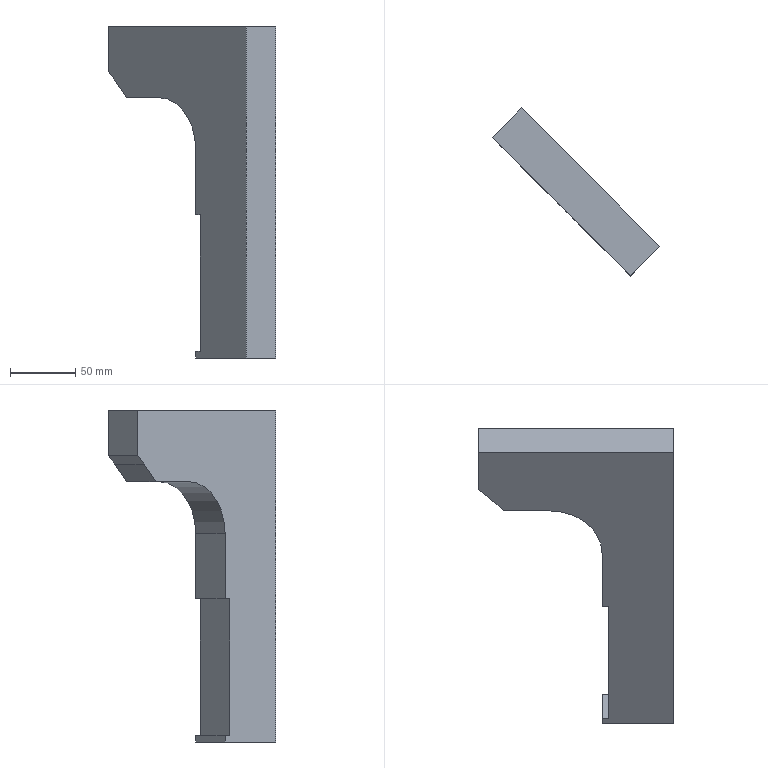Part | NX | features solid 2 | 1 solid | 15 faces | box 128.693 x 128.693 x 255 mm | volume 603628 mm3 | plane 14 | cylinder 1 | commonest cylinder face diameters 80 x1
STEP:
#1=CARTESIAN_POINT('',(803.273,-568.514,15.));
#2=VERTEX_POINT('',#1);
#3=CARTESIAN_POINT('',(803.273,-568.514,50.));
#4=VERTEX_POINT('',#3);
#5=CARTESIAN_POINT('',(803.273,-568.514,15.));
#6=DIRECTION('',(0.,0.,1.));
#7=VECTOR('',#6,1000.);
#8=LINE('',#5,#7);
#9=EDGE_CURVE('',#2,#4,#8,.T.);
#10=ORIENTED_EDGE('',*,*,#9,.F.);
#11=CARTESIAN_POINT('',(780.646,-591.141,15.));
#12=VERTEX_POINT('',#11);
#13=CARTESIAN_POINT('',(780.646,-591.141,15.));
#14=DIRECTION('',(0.7071,0.7071,0.));
#15=VECTOR('',#14,1000.);
#16=LINE('',#13,#15);
#17=EDGE_CURVE('',#12,#2,#16,.T.);
#18=ORIENTED_EDGE('',*,*,#17,.F.);
#19=CARTESIAN_POINT('',(780.646,-591.141,50.));
#20=VERTEX_POINT('',#19);
#21=CARTESIAN_POINT('',(780.646,-591.141,15.));
#22=DIRECTION('',(0.,0.,1.));
#23=VECTOR('',#22,1000.);
#24=LINE('',#21,#23);
#25=EDGE_CURVE('',#12,#20,#24,.T.);
#26=ORIENTED_EDGE('',*,*,#25,.T.);
#27=CARTESIAN_POINT('',(780.646,-591.141,50.));
#28=DIRECTION('',(0.7071,0.7071,0.));
#29=VECTOR('',#28,1000.);
#30=LINE('',#27,#29);
#31=EDGE_CURVE('',#20,#4,#30,.T.);
#32=ORIENTED_EDGE('',*,*,#31,.T.);
#33=EDGE_LOOP('',(#10,#18,#26,#32));
#34=FACE_BOUND('',#33,.T.);
#35=CARTESIAN_POINT('',(780.646,-591.141,15.));
#36=DIRECTION('',(-0.7071,0.7071,0.));
#37=DIRECTION('',(0.,0.,-1.));
#38=AXIS2_PLACEMENT_3D('',#35,#36,#37);
#39=PLANE('',#38);
#40=ADVANCED_FACE('',(#34),#39,.T.);
#41=CARTESIAN_POINT('',(808.223,-573.464,8.5));
#42=VERTEX_POINT('',#41);
#43=CARTESIAN_POINT('',(803.273,-568.514,15.));
#44=DIRECTION('',(0.5182,-0.5182,-0.6805));
#45=VECTOR('',#44,1000.);
#46=LINE('',#43,#45);
#47=EDGE_CURVE('',#2,#42,#46,.T.);
#48=ORIENTED_EDGE('',*,*,#47,.T.);
#49=CARTESIAN_POINT('',(785.596,-596.091,8.5));
#50=VERTEX_POINT('',#49);
#51=CARTESIAN_POINT('',(785.596,-596.091,8.5));
#52=DIRECTION('',(0.7071,0.7071,0.));
#53=VECTOR('',#52,1000.);
#54=LINE('',#51,#53);
#55=EDGE_CURVE('',#50,#42,#54,.T.);
#56=ORIENTED_EDGE('',*,*,#55,.F.);
#57=CARTESIAN_POINT('',(780.646,-591.141,15.));
#58=DIRECTION('',(0.5182,-0.5182,-0.6805));
#59=VECTOR('',#58,1000.);
#60=LINE('',#57,#59);
#61=EDGE_CURVE('',#12,#50,#60,.T.);
#62=ORIENTED_EDGE('',*,*,#61,.F.);
#63=ORIENTED_EDGE('',*,*,#17,.T.);
#64=EDGE_LOOP('',(#48,#56,#62,#63));
#65=FACE_BOUND('',#64,.T.);
#66=CARTESIAN_POINT('',(780.646,-591.141,15.));
#67=DIRECTION('',(0.4812,-0.4812,0.7328));
#68=DIRECTION('',(-0.5182,0.5182,0.6805));
#69=AXIS2_PLACEMENT_3D('',#66,#67,#68);
#70=PLANE('',#69);
#71=ADVANCED_FACE('',(#65),#70,.F.);
#72=CARTESIAN_POINT('',(817.415,-582.656,-5.));
#73=VERTEX_POINT('',#72);
#74=CARTESIAN_POINT('',(808.223,-573.464,8.5));
#75=DIRECTION('',(0.4905,-0.4905,-0.7203));
#76=VECTOR('',#75,1000.);
#77=LINE('',#74,#76);
#78=EDGE_CURVE('',#42,#73,#77,.T.);
#79=ORIENTED_EDGE('',*,*,#78,.T.);
#80=CARTESIAN_POINT('',(794.788,-605.283,-5.));
#81=VERTEX_POINT('',#80);
#82=CARTESIAN_POINT('',(794.788,-605.283,-5.));
#83=DIRECTION('',(0.7071,0.7071,0.));
#84=VECTOR('',#83,1000.);
#85=LINE('',#82,#84);
#86=EDGE_CURVE('',#81,#73,#85,.T.);
#87=ORIENTED_EDGE('',*,*,#86,.F.);
#88=CARTESIAN_POINT('',(785.596,-596.091,8.5));
#89=DIRECTION('',(0.4905,-0.4905,-0.7203));
#90=VECTOR('',#89,1000.);
#91=LINE('',#88,#90);
#92=EDGE_CURVE('',#50,#81,#91,.T.);
#93=ORIENTED_EDGE('',*,*,#92,.F.);
#94=ORIENTED_EDGE('',*,*,#55,.T.);
#95=EDGE_LOOP('',(#79,#87,#93,#94));
#96=FACE_BOUND('',#95,.T.);
#97=CARTESIAN_POINT('',(785.596,-596.091,8.5));
#98=DIRECTION('',(0.5093,-0.5093,0.6936));
#99=DIRECTION('',(-0.4905,0.4905,0.7203));
#100=AXIS2_PLACEMENT_3D('',#97,#98,#99);
#101=PLANE('',#100);
#102=ADVANCED_FACE('',(#96),#101,.F.);
#103=CARTESIAN_POINT('',(842.164,-607.405,-5.));
#104=VERTEX_POINT('',#103);
#105=CARTESIAN_POINT('',(817.415,-582.656,-5.));
#106=DIRECTION('',(0.7071,-0.7071,0.));
#107=VECTOR('',#106,1000.);
#108=LINE('',#105,#107);
#109=EDGE_CURVE('',#73,#104,#108,.T.);
#110=ORIENTED_EDGE('',*,*,#109,.T.);
#111=CARTESIAN_POINT('',(819.537,-630.032,-5.));
#112=VERTEX_POINT('',#111);
#113=CARTESIAN_POINT('',(819.537,-630.032,-5.));
#114=DIRECTION('',(0.7071,0.7071,0.));
#115=VECTOR('',#114,1000.);
#116=LINE('',#113,#115);
#117=EDGE_CURVE('',#112,#104,#116,.T.);
#118=ORIENTED_EDGE('',*,*,#117,.F.);
#119=CARTESIAN_POINT('',(794.788,-605.283,-5.));
#120=DIRECTION('',(0.7071,-0.7071,0.));
#121=VECTOR('',#120,1000.);
#122=LINE('',#119,#121);
#123=EDGE_CURVE('',#81,#112,#122,.T.);
#124=ORIENTED_EDGE('',*,*,#123,.F.);
#125=ORIENTED_EDGE('',*,*,#86,.T.);
#126=EDGE_LOOP('',(#110,#118,#124,#125));
#127=FACE_BOUND('',#126,.T.);
#128=CARTESIAN_POINT('',(794.788,-605.283,-5.));
#129=DIRECTION('',(0.,0.,1.));
#130=DIRECTION('',(-0.7071,0.7071,0.));
#131=AXIS2_PLACEMENT_3D('',#128,#129,#130);
#132=PLANE('',#131);
#133=ADVANCED_FACE('',(#127),#132,.F.);
#134=CARTESIAN_POINT('',(870.448,-635.689,-45.));
#135=VERTEX_POINT('',#134);
#136=CARTESIAN_POINT('',(842.164,-607.405,-45.));
#137=DIRECTION('',(-0.7071,-0.7071,0.));
#138=DIRECTION('',(0.7071,-0.7071,0.));
#139=AXIS2_PLACEMENT_3D('',#136,#137,#138);
#140=CIRCLE('',#139,40.);
#141=EDGE_CURVE('',#135,#104,#140,.T.);
#142=ORIENTED_EDGE('',*,*,#141,.F.);
#143=CARTESIAN_POINT('',(847.821,-658.316,-45.));
#144=VERTEX_POINT('',#143);
#145=CARTESIAN_POINT('',(847.821,-658.316,-45.));
#146=DIRECTION('',(0.7071,0.7071,0.));
#147=VECTOR('',#146,1000.);
#148=LINE('',#145,#147);
#149=EDGE_CURVE('',#144,#135,#148,.T.);
#150=ORIENTED_EDGE('',*,*,#149,.F.);
#151=CARTESIAN_POINT('',(819.537,-630.032,-45.));
#152=DIRECTION('',(-0.7071,-0.7071,0.));
#153=DIRECTION('',(0.7071,-0.7071,0.));
#154=AXIS2_PLACEMENT_3D('',#151,#152,#153);
#155=CIRCLE('',#154,40.);
#156=EDGE_CURVE('',#144,#112,#155,.T.);
#157=ORIENTED_EDGE('',*,*,#156,.T.);
#158=ORIENTED_EDGE('',*,*,#117,.T.);
#159=EDGE_LOOP('',(#142,#150,#157,#158));
#160=FACE_BOUND('',#159,.T.);
#161=CARTESIAN_POINT('',(819.537,-630.032,-45.));
#162=DIRECTION('',(0.7071,0.7071,0.));
#163=DIRECTION('',(0.,0.,-1.));
#164=AXIS2_PLACEMENT_3D('',#161,#162,#163);
#165=CYLINDRICAL_SURFACE('',#164,40.);
#166=ADVANCED_FACE('',(#160),#165,.F.);
#167=CARTESIAN_POINT('',(870.448,-635.689,-95.));
#168=VERTEX_POINT('',#167);
#169=CARTESIAN_POINT('',(870.448,-635.689,-45.));
#170=DIRECTION('',(0.,0.,-1.));
#171=VECTOR('',#170,1000.);
#172=LINE('',#169,#171);
#173=EDGE_CURVE('',#135,#168,#172,.T.);
#174=ORIENTED_EDGE('',*,*,#173,.T.);
#175=CARTESIAN_POINT('',(847.821,-658.316,-95.));
#176=VERTEX_POINT('',#175);
#177=CARTESIAN_POINT('',(847.821,-658.316,-95.));
#178=DIRECTION('',(0.7071,0.7071,0.));
#179=VECTOR('',#178,1000.);
#180=LINE('',#177,#179);
#181=EDGE_CURVE('',#176,#168,#180,.T.);
#182=ORIENTED_EDGE('',*,*,#181,.F.);
#183=CARTESIAN_POINT('',(847.821,-658.316,-45.));
#184=DIRECTION('',(0.,0.,-1.));
#185=VECTOR('',#184,1000.);
#186=LINE('',#183,#185);
#187=EDGE_CURVE('',#144,#176,#186,.T.);
#188=ORIENTED_EDGE('',*,*,#187,.F.);
#189=ORIENTED_EDGE('',*,*,#149,.T.);
#190=EDGE_LOOP('',(#174,#182,#188,#189));
#191=FACE_BOUND('',#190,.T.);
#192=CARTESIAN_POINT('',(847.821,-658.316,-45.));
#193=DIRECTION('',(0.7071,-0.7071,0.));
#194=DIRECTION('',(0.,0.,1.));
#195=AXIS2_PLACEMENT_3D('',#192,#193,#194);
#196=PLANE('',#195);
#197=ADVANCED_FACE('',(#191),#196,.F.);
#198=CARTESIAN_POINT('',(873.984,-639.225,-95.));
#199=VERTEX_POINT('',#198);
#200=CARTESIAN_POINT('',(863.377,-628.618,-95.));
#201=DIRECTION('',(0.7071,-0.7071,0.));
#202=VECTOR('',#201,1000.);
#203=LINE('',#200,#202);
#204=EDGE_CURVE('',#168,#199,#203,.T.);
#205=ORIENTED_EDGE('',*,*,#204,.T.);
#206=CARTESIAN_POINT('',(851.357,-661.852,-95.));
#207=VERTEX_POINT('',#206);
#208=CARTESIAN_POINT('',(851.357,-661.852,-95.));
#209=DIRECTION('',(0.7071,0.7071,0.));
#210=VECTOR('',#209,1000.);
#211=LINE('',#208,#210);
#212=EDGE_CURVE('',#207,#199,#211,.T.);
#213=ORIENTED_EDGE('',*,*,#212,.F.);
#214=CARTESIAN_POINT('',(840.75,-651.245,-95.));
#215=DIRECTION('',(0.7071,-0.7071,0.));
#216=VECTOR('',#215,1000.);
#217=LINE('',#214,#216);
#218=EDGE_CURVE('',#176,#207,#217,.T.);
#219=ORIENTED_EDGE('',*,*,#218,.F.);
#220=ORIENTED_EDGE('',*,*,#181,.T.);
#221=EDGE_LOOP('',(#205,#213,#219,#220));
#222=FACE_BOUND('',#221,.T.);
#223=CARTESIAN_POINT('',(840.75,-651.245,-95.));
#224=DIRECTION('',(0.,0.,1.));
#225=DIRECTION('',(-0.7071,0.7071,0.));
#226=AXIS2_PLACEMENT_3D('',#223,#224,#225);
#227=PLANE('',#226);
#228=ADVANCED_FACE('',(#222),#227,.F.);
#229=CARTESIAN_POINT('',(873.984,-639.225,-200.));
#230=VERTEX_POINT('',#229);
#231=CARTESIAN_POINT('',(873.984,-639.225,-95.));
#232=DIRECTION('',(0.,0.,-1.));
#233=VECTOR('',#232,1000.);
#234=LINE('',#231,#233);
#235=EDGE_CURVE('',#199,#230,#234,.T.);
#236=ORIENTED_EDGE('',*,*,#235,.T.);
#237=CARTESIAN_POINT('',(851.357,-661.852,-200.));
#238=VERTEX_POINT('',#237);
#239=CARTESIAN_POINT('',(851.357,-661.852,-200.));
#240=DIRECTION('',(0.7071,0.7071,0.));
#241=VECTOR('',#240,1000.);
#242=LINE('',#239,#241);
#243=EDGE_CURVE('',#238,#230,#242,.T.);
#244=ORIENTED_EDGE('',*,*,#243,.F.);
#245=CARTESIAN_POINT('',(851.357,-661.852,-95.));
#246=DIRECTION('',(0.,0.,-1.));
#247=VECTOR('',#246,1000.);
#248=LINE('',#245,#247);
#249=EDGE_CURVE('',#207,#238,#248,.T.);
#250=ORIENTED_EDGE('',*,*,#249,.F.);
#251=ORIENTED_EDGE('',*,*,#212,.T.);
#252=EDGE_LOOP('',(#236,#244,#250,#251));
#253=FACE_BOUND('',#252,.T.);
#254=CARTESIAN_POINT('',(851.357,-661.852,-95.));
#255=DIRECTION('',(0.7071,-0.7071,0.));
#256=DIRECTION('',(0.,0.,1.));
#257=AXIS2_PLACEMENT_3D('',#254,#255,#256);
#258=PLANE('',#257);
#259=ADVANCED_FACE('',(#253),#258,.F.);
#260=CARTESIAN_POINT('',(870.448,-635.689,-200.));
#261=VERTEX_POINT('',#260);
#262=CARTESIAN_POINT('',(873.984,-639.225,-200.));
#263=DIRECTION('',(-0.7071,0.7071,0.));
#264=VECTOR('',#263,1000.);
#265=LINE('',#262,#264);
#266=EDGE_CURVE('',#230,#261,#265,.T.);
#267=ORIENTED_EDGE('',*,*,#266,.T.);
#268=CARTESIAN_POINT('',(847.821,-658.316,-200.));
#269=VERTEX_POINT('',#268);
#270=CARTESIAN_POINT('',(847.821,-658.316,-200.));
#271=DIRECTION('',(0.7071,0.7071,0.));
#272=VECTOR('',#271,1000.);
#273=LINE('',#270,#272);
#274=EDGE_CURVE('',#269,#261,#273,.T.);
#275=ORIENTED_EDGE('',*,*,#274,.F.);
#276=CARTESIAN_POINT('',(851.357,-661.852,-200.));
#277=DIRECTION('',(-0.7071,0.7071,0.));
#278=VECTOR('',#277,1000.);
#279=LINE('',#276,#278);
#280=EDGE_CURVE('',#238,#269,#279,.T.);
#281=ORIENTED_EDGE('',*,*,#280,.F.);
#282=ORIENTED_EDGE('',*,*,#243,.T.);
#283=EDGE_LOOP('',(#267,#275,#281,#282));
#284=FACE_BOUND('',#283,.T.);
#285=CARTESIAN_POINT('',(851.357,-661.852,-200.));
#286=DIRECTION('',(0.,0.,-1.));
#287=DIRECTION('',(0.7071,-0.7071,0.));
#288=AXIS2_PLACEMENT_3D('',#285,#286,#287);
#289=PLANE('',#288);
#290=ADVANCED_FACE('',(#284),#289,.F.);
#291=CARTESIAN_POINT('',(870.448,-635.689,-205.));
#292=VERTEX_POINT('',#291);
#293=CARTESIAN_POINT('',(870.448,-635.689,-200.));
#294=DIRECTION('',(0.,0.,-1.));
#295=VECTOR('',#294,1000.);
#296=LINE('',#293,#295);
#297=EDGE_CURVE('',#261,#292,#296,.T.);
#298=ORIENTED_EDGE('',*,*,#297,.T.);
#299=CARTESIAN_POINT('',(847.821,-658.316,-205.));
#300=VERTEX_POINT('',#299);
#301=CARTESIAN_POINT('',(847.821,-658.316,-205.));
#302=DIRECTION('',(0.7071,0.7071,0.));
#303=VECTOR('',#302,1000.);
#304=LINE('',#301,#303);
#305=EDGE_CURVE('',#300,#292,#304,.T.);
#306=ORIENTED_EDGE('',*,*,#305,.F.);
#307=CARTESIAN_POINT('',(847.821,-658.316,-200.));
#308=DIRECTION('',(0.,0.,-1.));
#309=VECTOR('',#308,1000.);
#310=LINE('',#307,#309);
#311=EDGE_CURVE('',#269,#300,#310,.T.);
#312=ORIENTED_EDGE('',*,*,#311,.F.);
#313=ORIENTED_EDGE('',*,*,#274,.T.);
#314=EDGE_LOOP('',(#298,#306,#312,#313));
#315=FACE_BOUND('',#314,.T.);
#316=CARTESIAN_POINT('',(847.821,-658.316,-200.));
#317=DIRECTION('',(0.7071,-0.7071,0.));
#318=DIRECTION('',(0.,0.,1.));
#319=AXIS2_PLACEMENT_3D('',#316,#317,#318);
#320=PLANE('',#319);
#321=ADVANCED_FACE('',(#315),#320,.F.);
#322=CARTESIAN_POINT('',(909.339,-674.58,-205.));
#323=VERTEX_POINT('',#322);
#324=CARTESIAN_POINT('',(870.448,-635.689,-205.));
#325=DIRECTION('',(0.7071,-0.7071,0.));
#326=VECTOR('',#325,1000.);
#327=LINE('',#324,#326);
#328=EDGE_CURVE('',#292,#323,#327,.T.);
#329=ORIENTED_EDGE('',*,*,#328,.T.);
#330=CARTESIAN_POINT('',(886.712,-697.207,-205.));
#331=VERTEX_POINT('',#330);
#332=CARTESIAN_POINT('',(886.712,-697.207,-205.));
#333=DIRECTION('',(0.7071,0.7071,0.));
#334=VECTOR('',#333,1000.);
#335=LINE('',#332,#334);
#336=EDGE_CURVE('',#331,#323,#335,.T.);
#337=ORIENTED_EDGE('',*,*,#336,.F.);
#338=CARTESIAN_POINT('',(847.821,-658.316,-205.));
#339=DIRECTION('',(0.7071,-0.7071,0.));
#340=VECTOR('',#339,1000.);
#341=LINE('',#338,#340);
#342=EDGE_CURVE('',#300,#331,#341,.T.);
#343=ORIENTED_EDGE('',*,*,#342,.F.);
#344=ORIENTED_EDGE('',*,*,#305,.T.);
#345=EDGE_LOOP('',(#329,#337,#343,#344));
#346=FACE_BOUND('',#345,.T.);
#347=CARTESIAN_POINT('',(847.821,-658.316,-205.));
#348=DIRECTION('',(0.,0.,1.));
#349=DIRECTION('',(-0.7071,0.7071,0.));
#350=AXIS2_PLACEMENT_3D('',#347,#348,#349);
#351=PLANE('',#350);
#352=ADVANCED_FACE('',(#346),#351,.F.);
#353=CARTESIAN_POINT('',(909.339,-674.58,50.));
#354=VERTEX_POINT('',#353);
#355=CARTESIAN_POINT('',(909.339,-674.58,-205.));
#356=DIRECTION('',(0.,0.,1.));
#357=VECTOR('',#356,1000.);
#358=LINE('',#355,#357);
#359=EDGE_CURVE('',#323,#354,#358,.T.);
#360=ORIENTED_EDGE('',*,*,#359,.T.);
#361=CARTESIAN_POINT('',(886.712,-697.207,50.));
#362=VERTEX_POINT('',#361);
#363=CARTESIAN_POINT('',(886.712,-697.207,50.));
#364=DIRECTION('',(0.7071,0.7071,0.));
#365=VECTOR('',#364,1000.);
#366=LINE('',#363,#365);
#367=EDGE_CURVE('',#362,#354,#366,.T.);
#368=ORIENTED_EDGE('',*,*,#367,.F.);
#369=CARTESIAN_POINT('',(886.712,-697.207,-205.));
#370=DIRECTION('',(0.,0.,1.));
#371=VECTOR('',#370,1000.);
#372=LINE('',#369,#371);
#373=EDGE_CURVE('',#331,#362,#372,.T.);
#374=ORIENTED_EDGE('',*,*,#373,.F.);
#375=ORIENTED_EDGE('',*,*,#336,.T.);
#376=EDGE_LOOP('',(#360,#368,#374,#375));
#377=FACE_BOUND('',#376,.T.);
#378=CARTESIAN_POINT('',(886.712,-697.207,-205.));
#379=DIRECTION('',(-0.7071,0.7071,0.));
#380=DIRECTION('',(0.,0.,-1.));
#381=AXIS2_PLACEMENT_3D('',#378,#379,#380);
#382=PLANE('',#381);
#383=ADVANCED_FACE('',(#377),#382,.F.);
#384=CARTESIAN_POINT('',(771.454,-536.694,50.));
#385=DIRECTION('',(0.7071,-0.7071,0.));
#386=VECTOR('',#385,1000.);
#387=LINE('',#384,#386);
#388=EDGE_CURVE('',#4,#354,#387,.T.);
#389=ORIENTED_EDGE('',*,*,#388,.F.);
#390=ORIENTED_EDGE('',*,*,#31,.F.);
#391=CARTESIAN_POINT('',(748.826,-559.321,50.));
#392=DIRECTION('',(0.7071,-0.7071,0.));
#393=VECTOR('',#392,1000.);
#394=LINE('',#391,#393);
#395=EDGE_CURVE('',#20,#362,#394,.T.);
#396=ORIENTED_EDGE('',*,*,#395,.T.);
#397=ORIENTED_EDGE('',*,*,#367,.T.);
#398=EDGE_LOOP('',(#389,#390,#396,#397));
#399=FACE_BOUND('',#398,.T.);
#400=CARTESIAN_POINT('',(748.826,-559.321,50.));
#401=DIRECTION('',(0.,0.,1.));
#402=DIRECTION('',(-0.7071,0.7071,0.));
#403=AXIS2_PLACEMENT_3D('',#400,#401,#402);
#404=PLANE('',#403);
#405=ADVANCED_FACE('',(#399),#404,.T.);
#406=ORIENTED_EDGE('',*,*,#25,.F.);
#407=ORIENTED_EDGE('',*,*,#61,.T.);
#408=ORIENTED_EDGE('',*,*,#92,.T.);
#409=ORIENTED_EDGE('',*,*,#123,.T.);
#410=ORIENTED_EDGE('',*,*,#156,.F.);
#411=ORIENTED_EDGE('',*,*,#187,.T.);
#412=ORIENTED_EDGE('',*,*,#218,.T.);
#413=ORIENTED_EDGE('',*,*,#249,.T.);
#414=ORIENTED_EDGE('',*,*,#280,.T.);
#415=ORIENTED_EDGE('',*,*,#311,.T.);
#416=ORIENTED_EDGE('',*,*,#342,.T.);
#417=ORIENTED_EDGE('',*,*,#373,.T.);
#418=ORIENTED_EDGE('',*,*,#395,.F.);
#419=EDGE_LOOP('',(#406,#407,#408,#409,#410,#411,#412,#413,#414,#415,#416,#417,#418));
#420=FACE_BOUND('',#419,.T.);
#421=CARTESIAN_POINT('',(824.239,-634.735,-76.301));
#422=DIRECTION('',(-0.7071,-0.7071,0.));
#423=DIRECTION('',(0.,0.,1.));
#424=AXIS2_PLACEMENT_3D('',#421,#422,#423);
#425=PLANE('',#424);
#426=ADVANCED_FACE('',(#420),#425,.T.);
#427=ORIENTED_EDGE('',*,*,#9,.T.);
#428=ORIENTED_EDGE('',*,*,#388,.T.);
#429=ORIENTED_EDGE('',*,*,#359,.F.);
#430=ORIENTED_EDGE('',*,*,#328,.F.);
#431=ORIENTED_EDGE('',*,*,#297,.F.);
#432=ORIENTED_EDGE('',*,*,#266,.F.);
#433=ORIENTED_EDGE('',*,*,#235,.F.);
#434=ORIENTED_EDGE('',*,*,#204,.F.);
#435=ORIENTED_EDGE('',*,*,#173,.F.);
#436=ORIENTED_EDGE('',*,*,#141,.T.);
#437=ORIENTED_EDGE('',*,*,#109,.F.);
#438=ORIENTED_EDGE('',*,*,#78,.F.);
#439=ORIENTED_EDGE('',*,*,#47,.F.);
#440=EDGE_LOOP('',(#427,#428,#429,#430,#431,#432,#433,#434,#435,#436,#437,#438,#439));
#441=FACE_BOUND('',#440,.T.);
#442=CARTESIAN_POINT('',(846.867,-612.107,-76.301));
#443=DIRECTION('',(-0.7071,-0.7071,0.));
#444=DIRECTION('',(0.,0.,1.));
#445=AXIS2_PLACEMENT_3D('',#442,#443,#444);
#446=PLANE('',#445);
#447=ADVANCED_FACE('',(#441),#446,.F.);
#448=CLOSED_SHELL('',(#40,#71,#102,#133,#166,#197,#228,#259,#290,#321,#352,#383,#405,#426,#447));
#449=MANIFOLD_SOLID_BREP('',#448);
#450=(LENGTH_UNIT()NAMED_UNIT(*)SI_UNIT(.MILLI.,.METRE.));
#451=UNCERTAINTY_MEASURE_WITH_UNIT(LENGTH_MEASURE(0.00001),#450,'','');
#452=(NAMED_UNIT(*)PLANE_ANGLE_UNIT()SI_UNIT($,.RADIAN.));
#453=(NAMED_UNIT(*)SI_UNIT($,.STERADIAN.)SOLID_ANGLE_UNIT());
#454=(GEOMETRIC_REPRESENTATION_CONTEXT(3)GLOBAL_UNCERTAINTY_ASSIGNED_CONTEXT((#451))GLOBAL_UNIT_ASSIGNED_CONTEXT((#450,#452,#453))REPRESENTATION_CONTEXT('',''));
#455=ADVANCED_BREP_SHAPE_REPRESENTATION('',(#449),#454);